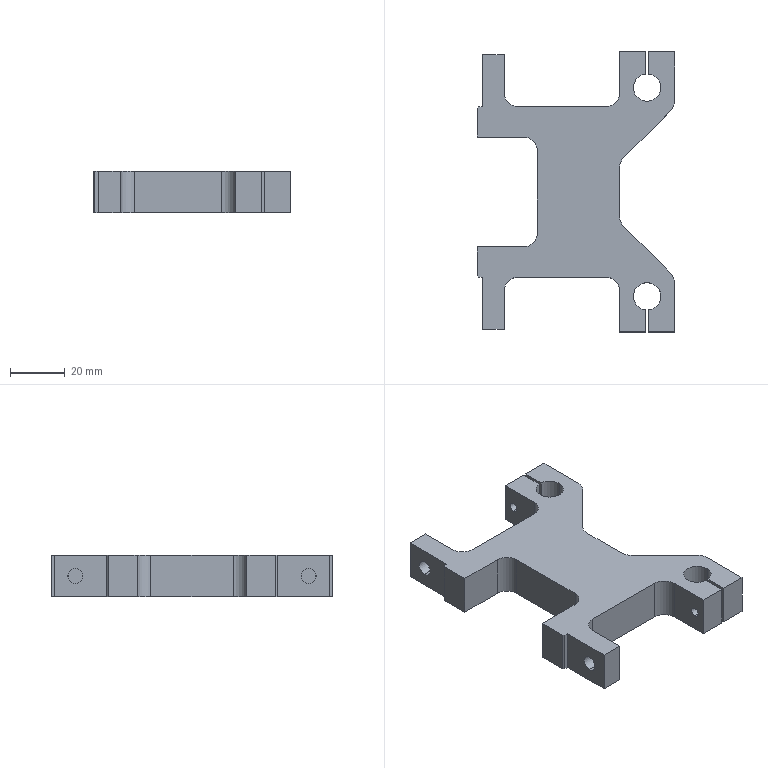Part | SolidWorks | features ICE 12, 3DProfileFeature 2, Chamfer 2, HoleWzd 2, Extrusion 1, Fillet 1 | 1 solid | 62 faces | box 71.8 x 102 x 15 mm | volume 54692 mm3 | plane 34 | cylinder 28 | commonest cylinder face diameters 10 x16 3.3 x4 4.5 x4 5.5 x4